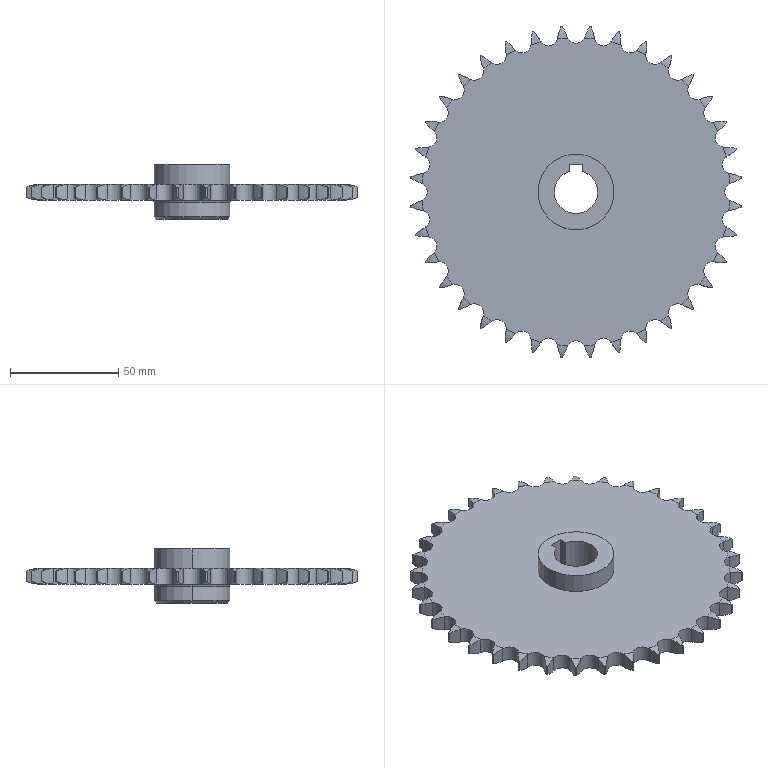Part | SolidWorks | features BaseBody 1 | 1 solid | 237 faces | box 152.556 x 152.556 x 25 mm | volume 123348 mm3 | cylinder 151 | torus 74 | plane 7 | cone 5 | commonest cylinder face diameters 77.611 x72 8.595 x36 153.081 x36 35 x4 20 x3